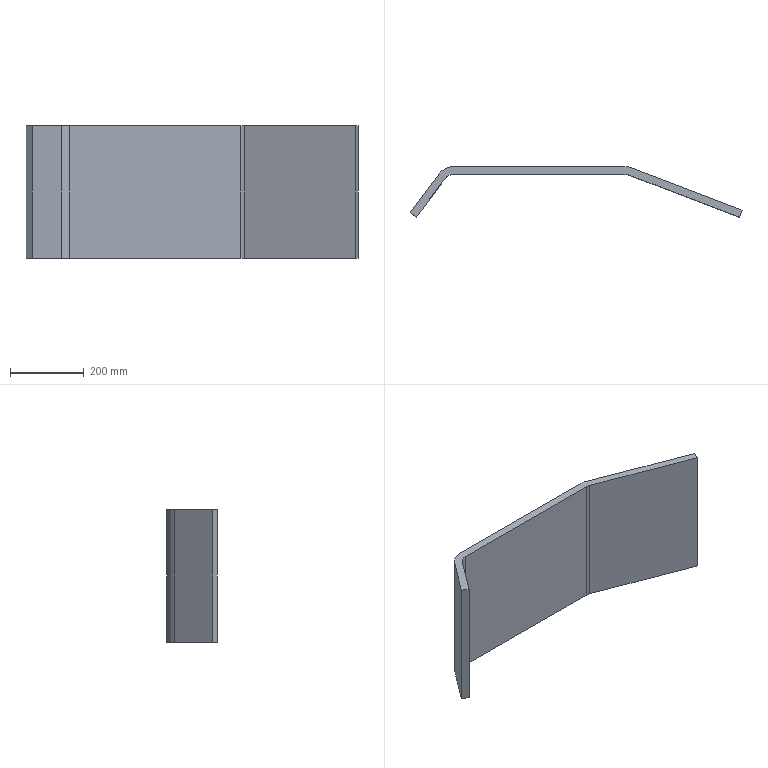Part | NX | features 底座(默认<按焊接>) 2 | 1 solid | 14 faces | box 901.587 x 137.68 x 360 mm | volume 7322251 mm3 | plane 10 | cylinder 4 | commonest cylinder face diameters 60 x2 102 x2
STEP:
#1=CARTESIAN_POINT('',(3031.433,684.,-26.));
#2=VERTEX_POINT('',#1);
#3=CARTESIAN_POINT('',(3042.161,682.016,-26.));
#4=VERTEX_POINT('',#3);
#5=CARTESIAN_POINT('',(3031.433,654.,-26.));
#6=DIRECTION('',(0.,0.,-1.));
#7=DIRECTION('',(-1.,0.,0.));
#8=AXIS2_PLACEMENT_3D('',#5,#6,#7);
#9=CIRCLE('',#8,30.);
#10=EDGE_CURVE('',#2,#4,#9,.T.);
#11=ORIENTED_EDGE('',*,*,#10,.F.);
#12=CARTESIAN_POINT('',(3031.433,684.,-386.));
#13=VERTEX_POINT('',#12);
#14=CARTESIAN_POINT('',(3031.433,684.,-386.));
#15=DIRECTION('',(0.,0.,1.));
#16=VECTOR('',#15,1000.);
#17=LINE('',#14,#16);
#18=EDGE_CURVE('',#13,#2,#17,.T.);
#19=ORIENTED_EDGE('',*,*,#18,.F.);
#20=CARTESIAN_POINT('',(3042.161,682.016,-386.));
#21=VERTEX_POINT('',#20);
#22=CARTESIAN_POINT('',(3031.433,654.,-386.));
#23=DIRECTION('',(0.,0.,-1.));
#24=DIRECTION('',(-1.,0.,0.));
#25=AXIS2_PLACEMENT_3D('',#22,#23,#24);
#26=CIRCLE('',#25,30.);
#27=EDGE_CURVE('',#13,#21,#26,.T.);
#28=ORIENTED_EDGE('',*,*,#27,.T.);
#29=CARTESIAN_POINT('',(3042.161,682.016,-386.));
#30=DIRECTION('',(0.,0.,1.));
#31=VECTOR('',#30,1000.);
#32=LINE('',#29,#31);
#33=EDGE_CURVE('',#21,#4,#32,.T.);
#34=ORIENTED_EDGE('',*,*,#33,.T.);
#35=EDGE_LOOP('',(#11,#19,#28,#34));
#36=FACE_BOUND('',#35,.T.);
#37=CARTESIAN_POINT('',(3031.433,654.,-386.));
#38=DIRECTION('',(0.,0.,1.));
#39=DIRECTION('',(1.,0.,0.));
#40=AXIS2_PLACEMENT_3D('',#37,#38,#39);
#41=CYLINDRICAL_SURFACE('',#40,30.);
#42=ADVANCED_FACE('',(#36),#41,.F.);
#43=CARTESIAN_POINT('',(2566.711,684.,-26.));
#44=VERTEX_POINT('',#43);
#45=CARTESIAN_POINT('',(3031.433,684.,-26.));
#46=DIRECTION('',(-1.,0.,0.));
#47=VECTOR('',#46,1000.);
#48=LINE('',#45,#47);
#49=EDGE_CURVE('',#2,#44,#48,.T.);
#50=ORIENTED_EDGE('',*,*,#49,.T.);
#51=CARTESIAN_POINT('',(2566.711,684.,-386.));
#52=VERTEX_POINT('',#51);
#53=CARTESIAN_POINT('',(2566.711,684.,-386.));
#54=DIRECTION('',(0.,0.,1.));
#55=VECTOR('',#54,1000.);
#56=LINE('',#53,#55);
#57=EDGE_CURVE('',#52,#44,#56,.T.);
#58=ORIENTED_EDGE('',*,*,#57,.F.);
#59=CARTESIAN_POINT('',(3031.433,684.,-386.));
#60=DIRECTION('',(-1.,0.,0.));
#61=VECTOR('',#60,1000.);
#62=LINE('',#59,#61);
#63=EDGE_CURVE('',#13,#52,#62,.T.);
#64=ORIENTED_EDGE('',*,*,#63,.F.);
#65=ORIENTED_EDGE('',*,*,#18,.T.);
#66=EDGE_LOOP('',(#50,#58,#64,#65));
#67=FACE_BOUND('',#66,.T.);
#68=CARTESIAN_POINT('',(3031.433,684.,-386.));
#69=DIRECTION('',(0.,1.,0.));
#70=DIRECTION('',(0.,0.,1.));
#71=AXIS2_PLACEMENT_3D('',#68,#69,#70);
#72=PLANE('',#71);
#73=ADVANCED_FACE('',(#67),#72,.F.);
#74=CARTESIAN_POINT('',(2542.686,671.967,-26.));
#75=VERTEX_POINT('',#74);
#76=CARTESIAN_POINT('',(2566.711,654.,-26.));
#77=DIRECTION('',(0.,0.,1.));
#78=DIRECTION('',(1.,0.,0.));
#79=AXIS2_PLACEMENT_3D('',#76,#77,#78);
#80=CIRCLE('',#79,30.);
#81=EDGE_CURVE('',#44,#75,#80,.T.);
#82=ORIENTED_EDGE('',*,*,#81,.T.);
#83=CARTESIAN_POINT('',(2542.686,671.967,-386.));
#84=VERTEX_POINT('',#83);
#85=CARTESIAN_POINT('',(2542.686,671.967,-386.));
#86=DIRECTION('',(0.,0.,1.));
#87=VECTOR('',#86,1000.);
#88=LINE('',#85,#87);
#89=EDGE_CURVE('',#84,#75,#88,.T.);
#90=ORIENTED_EDGE('',*,*,#89,.F.);
#91=CARTESIAN_POINT('',(2566.711,654.,-386.));
#92=DIRECTION('',(0.,0.,1.));
#93=DIRECTION('',(1.,0.,0.));
#94=AXIS2_PLACEMENT_3D('',#91,#92,#93);
#95=CIRCLE('',#94,30.);
#96=EDGE_CURVE('',#52,#84,#95,.T.);
#97=ORIENTED_EDGE('',*,*,#96,.F.);
#98=ORIENTED_EDGE('',*,*,#57,.T.);
#99=EDGE_LOOP('',(#82,#90,#97,#98));
#100=FACE_BOUND('',#99,.T.);
#101=CARTESIAN_POINT('',(2566.711,654.,-386.));
#102=DIRECTION('',(0.,0.,1.));
#103=DIRECTION('',(1.,0.,0.));
#104=AXIS2_PLACEMENT_3D('',#101,#102,#103);
#105=CYLINDRICAL_SURFACE('',#104,30.);
#106=ADVANCED_FACE('',(#100),#105,.F.);
#107=CARTESIAN_POINT('',(2464.425,567.32,-26.));
#108=VERTEX_POINT('',#107);
#109=CARTESIAN_POINT('',(2542.686,671.967,-26.));
#110=DIRECTION('',(-0.5989,-0.8008,0.));
#111=VECTOR('',#110,1000.);
#112=LINE('',#109,#111);
#113=EDGE_CURVE('',#75,#108,#112,.T.);
#114=ORIENTED_EDGE('',*,*,#113,.T.);
#115=CARTESIAN_POINT('',(2464.425,567.32,-386.));
#116=VERTEX_POINT('',#115);
#117=CARTESIAN_POINT('',(2464.425,567.32,-386.));
#118=DIRECTION('',(0.,0.,1.));
#119=VECTOR('',#118,1000.);
#120=LINE('',#117,#119);
#121=EDGE_CURVE('',#116,#108,#120,.T.);
#122=ORIENTED_EDGE('',*,*,#121,.F.);
#123=CARTESIAN_POINT('',(2542.686,671.967,-386.));
#124=DIRECTION('',(-0.5989,-0.8008,0.));
#125=VECTOR('',#124,1000.);
#126=LINE('',#123,#125);
#127=EDGE_CURVE('',#84,#116,#126,.T.);
#128=ORIENTED_EDGE('',*,*,#127,.F.);
#129=ORIENTED_EDGE('',*,*,#89,.T.);
#130=EDGE_LOOP('',(#114,#122,#128,#129));
#131=FACE_BOUND('',#130,.T.);
#132=CARTESIAN_POINT('',(2542.686,671.967,-386.));
#133=DIRECTION('',(-0.8008,0.5989,0.));
#134=DIRECTION('',(-0.5989,-0.8008,0.));
#135=AXIS2_PLACEMENT_3D('',#132,#133,#134);
#136=PLANE('',#135);
#137=ADVANCED_FACE('',(#131),#136,.F.);
#138=CARTESIAN_POINT('',(2447.608,579.897,-26.));
#139=VERTEX_POINT('',#138);
#140=CARTESIAN_POINT('',(2447.608,579.897,-26.));
#141=DIRECTION('',(0.8008,-0.5989,0.));
#142=VECTOR('',#141,1000.);
#143=LINE('',#140,#142);
#144=EDGE_CURVE('',#139,#108,#143,.T.);
#145=ORIENTED_EDGE('',*,*,#144,.F.);
#146=CARTESIAN_POINT('',(2447.608,579.897,-386.));
#147=VERTEX_POINT('',#146);
#148=CARTESIAN_POINT('',(2447.608,579.897,-386.));
#149=DIRECTION('',(0.,0.,1.));
#150=VECTOR('',#149,1000.);
#151=LINE('',#148,#150);
#152=EDGE_CURVE('',#147,#139,#151,.T.);
#153=ORIENTED_EDGE('',*,*,#152,.F.);
#154=CARTESIAN_POINT('',(2447.608,579.897,-386.));
#155=DIRECTION('',(0.8008,-0.5989,0.));
#156=VECTOR('',#155,1000.);
#157=LINE('',#154,#156);
#158=EDGE_CURVE('',#147,#116,#157,.T.);
#159=ORIENTED_EDGE('',*,*,#158,.T.);
#160=ORIENTED_EDGE('',*,*,#121,.T.);
#161=EDGE_LOOP('',(#145,#153,#159,#160));
#162=FACE_BOUND('',#161,.T.);
#163=CARTESIAN_POINT('',(2447.608,579.897,-386.));
#164=DIRECTION('',(-0.5989,-0.8008,0.));
#165=DIRECTION('',(0.8008,-0.5989,0.));
#166=AXIS2_PLACEMENT_3D('',#163,#164,#165);
#167=PLANE('',#166);
#168=ADVANCED_FACE('',(#162),#167,.T.);
#169=CARTESIAN_POINT('',(2525.869,684.544,-26.));
#170=VERTEX_POINT('',#169);
#171=CARTESIAN_POINT('',(2525.869,684.544,-26.));
#172=DIRECTION('',(-0.5989,-0.8008,0.));
#173=VECTOR('',#172,1000.);
#174=LINE('',#171,#173);
#175=EDGE_CURVE('',#170,#139,#174,.T.);
#176=ORIENTED_EDGE('',*,*,#175,.F.);
#177=CARTESIAN_POINT('',(2525.869,684.544,-386.));
#178=VERTEX_POINT('',#177);
#179=CARTESIAN_POINT('',(2525.869,684.544,-386.));
#180=DIRECTION('',(0.,0.,1.));
#181=VECTOR('',#180,1000.);
#182=LINE('',#179,#181);
#183=EDGE_CURVE('',#178,#170,#182,.T.);
#184=ORIENTED_EDGE('',*,*,#183,.F.);
#185=CARTESIAN_POINT('',(2525.869,684.544,-386.));
#186=DIRECTION('',(-0.5989,-0.8008,0.));
#187=VECTOR('',#186,1000.);
#188=LINE('',#185,#187);
#189=EDGE_CURVE('',#178,#147,#188,.T.);
#190=ORIENTED_EDGE('',*,*,#189,.T.);
#191=ORIENTED_EDGE('',*,*,#152,.T.);
#192=EDGE_LOOP('',(#176,#184,#190,#191));
#193=FACE_BOUND('',#192,.T.);
#194=CARTESIAN_POINT('',(2525.869,684.544,-386.));
#195=DIRECTION('',(-0.8008,0.5989,0.));
#196=DIRECTION('',(-0.5989,-0.8008,0.));
#197=AXIS2_PLACEMENT_3D('',#194,#195,#196);
#198=PLANE('',#197);
#199=ADVANCED_FACE('',(#193),#198,.T.);
#200=CARTESIAN_POINT('',(2566.711,705.,-26.));
#201=VERTEX_POINT('',#200);
#202=CARTESIAN_POINT('',(2566.711,654.,-26.));
#203=DIRECTION('',(0.,0.,1.));
#204=DIRECTION('',(1.,0.,0.));
#205=AXIS2_PLACEMENT_3D('',#202,#203,#204);
#206=CIRCLE('',#205,51.);
#207=EDGE_CURVE('',#201,#170,#206,.T.);
#208=ORIENTED_EDGE('',*,*,#207,.F.);
#209=CARTESIAN_POINT('',(2566.711,705.,-386.));
#210=VERTEX_POINT('',#209);
#211=CARTESIAN_POINT('',(2566.711,705.,-386.));
#212=DIRECTION('',(0.,0.,1.));
#213=VECTOR('',#212,1000.);
#214=LINE('',#211,#213);
#215=EDGE_CURVE('',#210,#201,#214,.T.);
#216=ORIENTED_EDGE('',*,*,#215,.F.);
#217=CARTESIAN_POINT('',(2566.711,654.,-386.));
#218=DIRECTION('',(0.,0.,1.));
#219=DIRECTION('',(1.,0.,0.));
#220=AXIS2_PLACEMENT_3D('',#217,#218,#219);
#221=CIRCLE('',#220,51.);
#222=EDGE_CURVE('',#210,#178,#221,.T.);
#223=ORIENTED_EDGE('',*,*,#222,.T.);
#224=ORIENTED_EDGE('',*,*,#183,.T.);
#225=EDGE_LOOP('',(#208,#216,#223,#224));
#226=FACE_BOUND('',#225,.T.);
#227=CARTESIAN_POINT('',(2566.711,654.,-386.));
#228=DIRECTION('',(0.,0.,1.));
#229=DIRECTION('',(1.,0.,0.));
#230=AXIS2_PLACEMENT_3D('',#227,#228,#229);
#231=CYLINDRICAL_SURFACE('',#230,51.);
#232=ADVANCED_FACE('',(#226),#231,.T.);
#233=CARTESIAN_POINT('',(3031.433,705.,-26.));
#234=VERTEX_POINT('',#233);
#235=CARTESIAN_POINT('',(3031.433,705.,-26.));
#236=DIRECTION('',(-1.,0.,0.));
#237=VECTOR('',#236,1000.);
#238=LINE('',#235,#237);
#239=EDGE_CURVE('',#234,#201,#238,.T.);
#240=ORIENTED_EDGE('',*,*,#239,.F.);
#241=CARTESIAN_POINT('',(3031.433,705.,-386.));
#242=VERTEX_POINT('',#241);
#243=CARTESIAN_POINT('',(3031.433,705.,-386.));
#244=DIRECTION('',(0.,0.,1.));
#245=VECTOR('',#244,1000.);
#246=LINE('',#243,#245);
#247=EDGE_CURVE('',#242,#234,#246,.T.);
#248=ORIENTED_EDGE('',*,*,#247,.F.);
#249=CARTESIAN_POINT('',(3031.433,705.,-386.));
#250=DIRECTION('',(-1.,0.,0.));
#251=VECTOR('',#250,1000.);
#252=LINE('',#249,#251);
#253=EDGE_CURVE('',#242,#210,#252,.T.);
#254=ORIENTED_EDGE('',*,*,#253,.T.);
#255=ORIENTED_EDGE('',*,*,#215,.T.);
#256=EDGE_LOOP('',(#240,#248,#254,#255));
#257=FACE_BOUND('',#256,.T.);
#258=CARTESIAN_POINT('',(3031.433,705.,-386.));
#259=DIRECTION('',(0.,1.,0.));
#260=DIRECTION('',(-1.,0.,0.));
#261=AXIS2_PLACEMENT_3D('',#258,#259,#260);
#262=PLANE('',#261);
#263=ADVANCED_FACE('',(#257),#262,.T.);
#264=CARTESIAN_POINT('',(3049.671,701.627,-26.));
#265=VERTEX_POINT('',#264);
#266=CARTESIAN_POINT('',(3031.433,654.,-26.));
#267=DIRECTION('',(0.,0.,-1.));
#268=DIRECTION('',(-1.,0.,0.));
#269=AXIS2_PLACEMENT_3D('',#266,#267,#268);
#270=CIRCLE('',#269,51.);
#271=EDGE_CURVE('',#234,#265,#270,.T.);
#272=ORIENTED_EDGE('',*,*,#271,.T.);
#273=CARTESIAN_POINT('',(3049.671,701.627,-386.));
#274=VERTEX_POINT('',#273);
#275=CARTESIAN_POINT('',(3049.671,701.627,-386.));
#276=DIRECTION('',(0.,0.,1.));
#277=VECTOR('',#276,1000.);
#278=LINE('',#275,#277);
#279=EDGE_CURVE('',#274,#265,#278,.T.);
#280=ORIENTED_EDGE('',*,*,#279,.F.);
#281=CARTESIAN_POINT('',(3031.433,654.,-386.));
#282=DIRECTION('',(0.,0.,-1.));
#283=DIRECTION('',(-1.,0.,0.));
#284=AXIS2_PLACEMENT_3D('',#281,#282,#283);
#285=CIRCLE('',#284,51.);
#286=EDGE_CURVE('',#242,#274,#285,.T.);
#287=ORIENTED_EDGE('',*,*,#286,.F.);
#288=ORIENTED_EDGE('',*,*,#247,.T.);
#289=EDGE_LOOP('',(#272,#280,#287,#288));
#290=FACE_BOUND('',#289,.T.);
#291=CARTESIAN_POINT('',(3031.433,654.,-386.));
#292=DIRECTION('',(0.,0.,1.));
#293=DIRECTION('',(1.,0.,0.));
#294=AXIS2_PLACEMENT_3D('',#291,#292,#293);
#295=CYLINDRICAL_SURFACE('',#294,51.);
#296=ADVANCED_FACE('',(#290),#295,.T.);
#297=CARTESIAN_POINT('',(3349.195,586.931,-26.));
#298=VERTEX_POINT('',#297);
#299=CARTESIAN_POINT('',(3049.671,701.627,-26.));
#300=DIRECTION('',(0.9339,-0.3576,0.));
#301=VECTOR('',#300,1000.);
#302=LINE('',#299,#301);
#303=EDGE_CURVE('',#265,#298,#302,.T.);
#304=ORIENTED_EDGE('',*,*,#303,.T.);
#305=CARTESIAN_POINT('',(3349.195,586.931,-386.));
#306=VERTEX_POINT('',#305);
#307=CARTESIAN_POINT('',(3349.195,586.931,-386.));
#308=DIRECTION('',(0.,0.,1.));
#309=VECTOR('',#308,1000.);
#310=LINE('',#307,#309);
#311=EDGE_CURVE('',#306,#298,#310,.T.);
#312=ORIENTED_EDGE('',*,*,#311,.F.);
#313=CARTESIAN_POINT('',(3049.671,701.627,-386.));
#314=DIRECTION('',(0.9339,-0.3576,0.));
#315=VECTOR('',#314,1000.);
#316=LINE('',#313,#315);
#317=EDGE_CURVE('',#274,#306,#316,.T.);
#318=ORIENTED_EDGE('',*,*,#317,.F.);
#319=ORIENTED_EDGE('',*,*,#279,.T.);
#320=EDGE_LOOP('',(#304,#312,#318,#319));
#321=FACE_BOUND('',#320,.T.);
#322=CARTESIAN_POINT('',(3049.671,701.627,-386.));
#323=DIRECTION('',(-0.3576,-0.9339,0.));
#324=DIRECTION('',(0.9339,-0.3576,0.));
#325=AXIS2_PLACEMENT_3D('',#322,#323,#324);
#326=PLANE('',#325);
#327=ADVANCED_FACE('',(#321),#326,.F.);
#328=CARTESIAN_POINT('',(3341.685,567.32,-26.));
#329=VERTEX_POINT('',#328);
#330=CARTESIAN_POINT('',(3341.685,567.32,-26.));
#331=DIRECTION('',(0.3576,0.9339,0.));
#332=VECTOR('',#331,1000.);
#333=LINE('',#330,#332);
#334=EDGE_CURVE('',#329,#298,#333,.T.);
#335=ORIENTED_EDGE('',*,*,#334,.F.);
#336=CARTESIAN_POINT('',(3341.685,567.32,-386.));
#337=VERTEX_POINT('',#336);
#338=CARTESIAN_POINT('',(3341.685,567.32,-386.));
#339=DIRECTION('',(0.,0.,1.));
#340=VECTOR('',#339,1000.);
#341=LINE('',#338,#340);
#342=EDGE_CURVE('',#337,#329,#341,.T.);
#343=ORIENTED_EDGE('',*,*,#342,.F.);
#344=CARTESIAN_POINT('',(3341.685,567.32,-386.));
#345=DIRECTION('',(0.3576,0.9339,0.));
#346=VECTOR('',#345,1000.);
#347=LINE('',#344,#346);
#348=EDGE_CURVE('',#337,#306,#347,.T.);
#349=ORIENTED_EDGE('',*,*,#348,.T.);
#350=ORIENTED_EDGE('',*,*,#311,.T.);
#351=EDGE_LOOP('',(#335,#343,#349,#350));
#352=FACE_BOUND('',#351,.T.);
#353=CARTESIAN_POINT('',(3341.685,567.32,-386.));
#354=DIRECTION('',(0.9339,-0.3576,0.));
#355=DIRECTION('',(0.3576,0.9339,0.));
#356=AXIS2_PLACEMENT_3D('',#353,#354,#355);
#357=PLANE('',#356);
#358=ADVANCED_FACE('',(#352),#357,.T.);
#359=CARTESIAN_POINT('',(3042.161,682.016,-26.));
#360=DIRECTION('',(0.9339,-0.3576,0.));
#361=VECTOR('',#360,1000.);
#362=LINE('',#359,#361);
#363=EDGE_CURVE('',#4,#329,#362,.T.);
#364=ORIENTED_EDGE('',*,*,#363,.F.);
#365=ORIENTED_EDGE('',*,*,#33,.F.);
#366=CARTESIAN_POINT('',(3042.161,682.016,-386.));
#367=DIRECTION('',(0.9339,-0.3576,0.));
#368=VECTOR('',#367,1000.);
#369=LINE('',#366,#368);
#370=EDGE_CURVE('',#21,#337,#369,.T.);
#371=ORIENTED_EDGE('',*,*,#370,.T.);
#372=ORIENTED_EDGE('',*,*,#342,.T.);
#373=EDGE_LOOP('',(#364,#365,#371,#372));
#374=FACE_BOUND('',#373,.T.);
#375=CARTESIAN_POINT('',(3042.161,682.016,-386.));
#376=DIRECTION('',(-0.3576,-0.9339,0.));
#377=DIRECTION('',(0.9339,-0.3576,0.));
#378=AXIS2_PLACEMENT_3D('',#375,#376,#377);
#379=PLANE('',#378);
#380=ADVANCED_FACE('',(#374),#379,.T.);
#381=ORIENTED_EDGE('',*,*,#27,.F.);
#382=ORIENTED_EDGE('',*,*,#63,.T.);
#383=ORIENTED_EDGE('',*,*,#96,.T.);
#384=ORIENTED_EDGE('',*,*,#127,.T.);
#385=ORIENTED_EDGE('',*,*,#158,.F.);
#386=ORIENTED_EDGE('',*,*,#189,.F.);
#387=ORIENTED_EDGE('',*,*,#222,.F.);
#388=ORIENTED_EDGE('',*,*,#253,.F.);
#389=ORIENTED_EDGE('',*,*,#286,.T.);
#390=ORIENTED_EDGE('',*,*,#317,.T.);
#391=ORIENTED_EDGE('',*,*,#348,.F.);
#392=ORIENTED_EDGE('',*,*,#370,.F.);
#393=EDGE_LOOP('',(#381,#382,#383,#384,#385,#386,#387,#388,#389,#390,#391,#392));
#394=FACE_BOUND('',#393,.T.);
#395=CARTESIAN_POINT('',(3031.433,654.,-386.));
#396=DIRECTION('',(0.,0.,-1.));
#397=DIRECTION('',(-1.,0.,0.));
#398=AXIS2_PLACEMENT_3D('',#395,#396,#397);
#399=PLANE('',#398);
#400=ADVANCED_FACE('',(#394),#399,.T.);
#401=ORIENTED_EDGE('',*,*,#10,.T.);
#402=ORIENTED_EDGE('',*,*,#363,.T.);
#403=ORIENTED_EDGE('',*,*,#334,.T.);
#404=ORIENTED_EDGE('',*,*,#303,.F.);
#405=ORIENTED_EDGE('',*,*,#271,.F.);
#406=ORIENTED_EDGE('',*,*,#239,.T.);
#407=ORIENTED_EDGE('',*,*,#207,.T.);
#408=ORIENTED_EDGE('',*,*,#175,.T.);
#409=ORIENTED_EDGE('',*,*,#144,.T.);
#410=ORIENTED_EDGE('',*,*,#113,.F.);
#411=ORIENTED_EDGE('',*,*,#81,.F.);
#412=ORIENTED_EDGE('',*,*,#49,.F.);
#413=EDGE_LOOP('',(#401,#402,#403,#404,#405,#406,#407,#408,#409,#410,#411,#412));
#414=FACE_BOUND('',#413,.T.);
#415=CARTESIAN_POINT('',(3031.433,654.,-26.));
#416=DIRECTION('',(0.,0.,-1.));
#417=DIRECTION('',(-1.,0.,0.));
#418=AXIS2_PLACEMENT_3D('',#415,#416,#417);
#419=PLANE('',#418);
#420=ADVANCED_FACE('',(#414),#419,.F.);
#421=CLOSED_SHELL('',(#42,#73,#106,#137,#168,#199,#232,#263,#296,#327,#358,#380,#400,#420));
#422=MANIFOLD_SOLID_BREP('',#421);
#423=(LENGTH_UNIT()NAMED_UNIT(*)SI_UNIT(.MILLI.,.METRE.));
#424=UNCERTAINTY_MEASURE_WITH_UNIT(LENGTH_MEASURE(0.00001),#423,'','');
#425=(NAMED_UNIT(*)PLANE_ANGLE_UNIT()SI_UNIT($,.RADIAN.));
#426=(NAMED_UNIT(*)SI_UNIT($,.STERADIAN.)SOLID_ANGLE_UNIT());
#427=(GEOMETRIC_REPRESENTATION_CONTEXT(3)GLOBAL_UNCERTAINTY_ASSIGNED_CONTEXT((#424))GLOBAL_UNIT_ASSIGNED_CONTEXT((#423,#425,#426))REPRESENTATION_CONTEXT('',''));
#428=ADVANCED_BREP_SHAPE_REPRESENTATION('',(#422),#427);